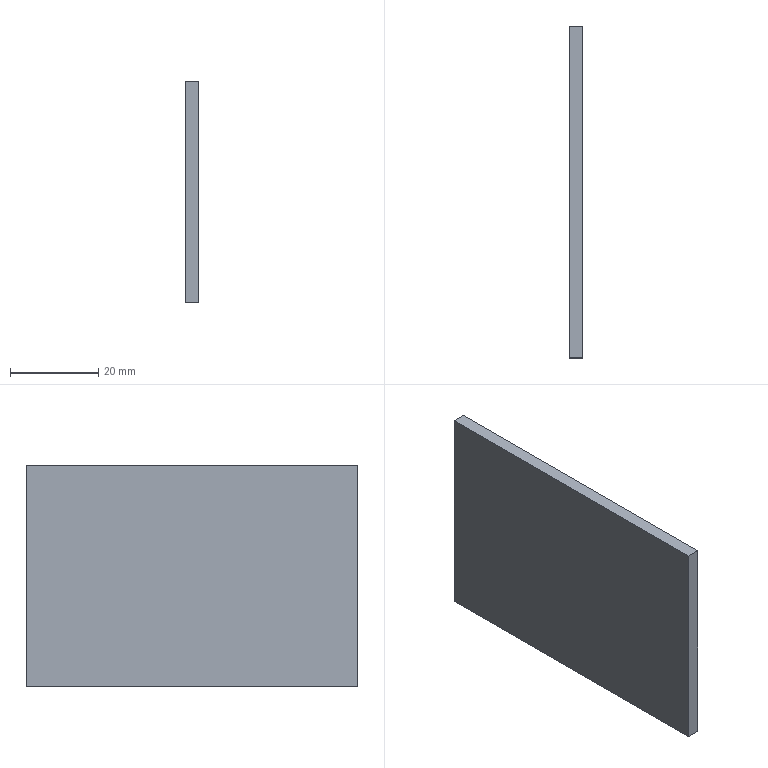Part | STEP file | Positioning_id1486_x_t | 1 solid | 6 faces | box 3 x 75 x 50 mm | volume 11250 mm3 | plane 6
STEP:
#1=CARTESIAN_POINT('',(0.,0.,0.));
#2=DIRECTION('',(0.,0.,1.));
#3=DIRECTION('',(1.,0.,0.));
#4=AXIS2_PLACEMENT_3D('',#1,#2,#3);
#5=CARTESIAN_POINT('',(-1013.002,-37.5,133.532));
#6=VERTEX_POINT('',#5);
#7=CARTESIAN_POINT('',(-1010.002,-37.5,133.532));
#8=VERTEX_POINT('',#7);
#9=CARTESIAN_POINT('',(-1013.002,-37.5,133.532));
#10=DIRECTION('',(1.,0.,0.));
#11=VECTOR('',#10,1.);
#12=LINE('',#9,#11);
#13=CARTESIAN_POINT('',(-1015.002,-37.5,143.532));
#14=DIRECTION('',(0.,-1.,0.));
#15=DIRECTION('',(1.,0.,0.));
#16=AXIS2_PLACEMENT_3D('',#13,#14,#15);
#17=PLANE('',#16);
#18=CARTESIAN_POINT('',(2.,-10.));
#19=DIRECTION('',(1.,0.));
#20=VECTOR('',#19,1.);
#21=LINE('',#18,#20);
#22=(GEOMETRIC_REPRESENTATION_CONTEXT(2)PARAMETRIC_REPRESENTATION_CONTEXT()REPRESENTATION_CONTEXT('',''));
#23=DEFINITIONAL_REPRESENTATION('',(#21),#22);
#24=PCURVE('',#17,#23);
#25=CARTESIAN_POINT('',(-1015.002,2.5,133.532));
#26=DIRECTION('',(0.,0.,-1.));
#27=DIRECTION('',(1.,0.,0.));
#28=AXIS2_PLACEMENT_3D('',#25,#26,#27);
#29=PLANE('',#28);
#30=CARTESIAN_POINT('',(2.,40.));
#31=DIRECTION('',(1.,0.));
#32=VECTOR('',#31,1.);
#33=LINE('',#30,#32);
#34=(GEOMETRIC_REPRESENTATION_CONTEXT(2)PARAMETRIC_REPRESENTATION_CONTEXT()REPRESENTATION_CONTEXT('',''));
#35=DEFINITIONAL_REPRESENTATION('',(#33),#34);
#36=PCURVE('',#29,#35);
#37=SURFACE_CURVE('',#12,(#24,#36),.PCURVE_S1.);
#38=EDGE_CURVE('',#6,#8,#37,.T.);
#39=ORIENTED_EDGE('',*,*,#38,.T.);
#40=CARTESIAN_POINT('',(-1010.002,-37.5,183.532));
#41=VERTEX_POINT('',#40);
#42=CARTESIAN_POINT('',(-1010.002,-37.5,133.532));
#43=DIRECTION('',(0.,0.,1.));
#44=VECTOR('',#43,1.);
#45=LINE('',#42,#44);
#46=CARTESIAN_POINT('',(5.,-10.));
#47=DIRECTION('',(0.,1.));
#48=VECTOR('',#47,1.);
#49=LINE('',#46,#48);
#50=(GEOMETRIC_REPRESENTATION_CONTEXT(2)PARAMETRIC_REPRESENTATION_CONTEXT()REPRESENTATION_CONTEXT('',''));
#51=DEFINITIONAL_REPRESENTATION('',(#49),#50);
#52=PCURVE('',#17,#51);
#53=CARTESIAN_POINT('',(-1010.002,-37.5,133.532));
#54=DIRECTION('',(1.,0.,0.));
#55=DIRECTION('',(0.,0.,1.));
#56=AXIS2_PLACEMENT_3D('',#53,#54,#55);
#57=PLANE('',#56);
#58=CARTESIAN_POINT('',(0.,0.));
#59=DIRECTION('',(1.,0.));
#60=VECTOR('',#59,1.);
#61=LINE('',#58,#60);
#62=(GEOMETRIC_REPRESENTATION_CONTEXT(2)PARAMETRIC_REPRESENTATION_CONTEXT()REPRESENTATION_CONTEXT('',''));
#63=DEFINITIONAL_REPRESENTATION('',(#61),#62);
#64=PCURVE('',#57,#63);
#65=SURFACE_CURVE('',#45,(#52,#64),.PCURVE_S1.);
#66=EDGE_CURVE('',#8,#41,#65,.T.);
#67=ORIENTED_EDGE('',*,*,#66,.T.);
#68=CARTESIAN_POINT('',(-1013.002,-37.5,183.532));
#69=VERTEX_POINT('',#68);
#70=CARTESIAN_POINT('',(-1013.002,-37.5,183.532));
#71=DIRECTION('',(1.,0.,0.));
#72=VECTOR('',#71,1.);
#73=LINE('',#70,#72);
#74=CARTESIAN_POINT('',(2.,40.));
#75=DIRECTION('',(1.,0.));
#76=VECTOR('',#75,1.);
#77=LINE('',#74,#76);
#78=(GEOMETRIC_REPRESENTATION_CONTEXT(2)PARAMETRIC_REPRESENTATION_CONTEXT()REPRESENTATION_CONTEXT('',''));
#79=DEFINITIONAL_REPRESENTATION('',(#77),#78);
#80=PCURVE('',#17,#79);
#81=CARTESIAN_POINT('',(-1015.002,2.5,183.532));
#82=DIRECTION('',(0.,0.,1.));
#83=DIRECTION('',(-1.,0.,0.));
#84=AXIS2_PLACEMENT_3D('',#81,#82,#83);
#85=PLANE('',#84);
#86=CARTESIAN_POINT('',(-2.,40.));
#87=DIRECTION('',(-1.,0.));
#88=VECTOR('',#87,1.);
#89=LINE('',#86,#88);
#90=(GEOMETRIC_REPRESENTATION_CONTEXT(2)PARAMETRIC_REPRESENTATION_CONTEXT()REPRESENTATION_CONTEXT('',''));
#91=DEFINITIONAL_REPRESENTATION('',(#89),#90);
#92=PCURVE('',#85,#91);
#93=SURFACE_CURVE('',#73,(#80,#92),.PCURVE_S1.);
#94=EDGE_CURVE('',#69,#41,#93,.T.);
#95=ORIENTED_EDGE('',*,*,#94,.F.);
#96=CARTESIAN_POINT('',(-1013.002,-37.5,183.532));
#97=DIRECTION('',(0.,0.,-1.));
#98=VECTOR('',#97,1.);
#99=LINE('',#96,#98);
#100=CARTESIAN_POINT('',(2.,40.));
#101=DIRECTION('',(0.,-1.));
#102=VECTOR('',#101,1.);
#103=LINE('',#100,#102);
#104=(GEOMETRIC_REPRESENTATION_CONTEXT(2)PARAMETRIC_REPRESENTATION_CONTEXT()REPRESENTATION_CONTEXT('',''));
#105=DEFINITIONAL_REPRESENTATION('',(#103),#104);
#106=PCURVE('',#17,#105);
#107=CARTESIAN_POINT('',(-1013.002,2.5,143.532));
#108=DIRECTION('',(-1.,0.,0.));
#109=DIRECTION('',(0.,0.,-1.));
#110=AXIS2_PLACEMENT_3D('',#107,#108,#109);
#111=PLANE('',#110);
#112=CARTESIAN_POINT('',(-40.,40.));
#113=DIRECTION('',(1.,0.));
#114=VECTOR('',#113,1.);
#115=LINE('',#112,#114);
#116=(GEOMETRIC_REPRESENTATION_CONTEXT(2)PARAMETRIC_REPRESENTATION_CONTEXT()REPRESENTATION_CONTEXT('',''));
#117=DEFINITIONAL_REPRESENTATION('',(#115),#116);
#118=PCURVE('',#111,#117);
#119=SURFACE_CURVE('',#99,(#106,#118),.PCURVE_S1.);
#120=EDGE_CURVE('',#69,#6,#119,.T.);
#121=ORIENTED_EDGE('',*,*,#120,.T.);
#122=EDGE_LOOP('',(#39,#67,#95,#121));
#123=FACE_BOUND('',#122,.T.);
#124=ADVANCED_FACE('',(#123),#17,.T.);
#125=ORIENTED_EDGE('',*,*,#94,.T.);
#126=CARTESIAN_POINT('',(-1010.002,37.5,183.532));
#127=VERTEX_POINT('',#126);
#128=CARTESIAN_POINT('',(-1010.002,-37.5,183.532));
#129=DIRECTION('',(0.,1.,0.));
#130=VECTOR('',#129,1.);
#131=LINE('',#128,#130);
#132=CARTESIAN_POINT('',(-5.,40.));
#133=DIRECTION('',(0.,-1.));
#134=VECTOR('',#133,1.);
#135=LINE('',#132,#134);
#136=(GEOMETRIC_REPRESENTATION_CONTEXT(2)PARAMETRIC_REPRESENTATION_CONTEXT()REPRESENTATION_CONTEXT('',''));
#137=DEFINITIONAL_REPRESENTATION('',(#135),#136);
#138=PCURVE('',#85,#137);
#139=CARTESIAN_POINT('',(50.,0.));
#140=DIRECTION('',(0.,-1.));
#141=VECTOR('',#140,1.);
#142=LINE('',#139,#141);
#143=(GEOMETRIC_REPRESENTATION_CONTEXT(2)PARAMETRIC_REPRESENTATION_CONTEXT()REPRESENTATION_CONTEXT('',''));
#144=DEFINITIONAL_REPRESENTATION('',(#142),#143);
#145=PCURVE('',#57,#144);
#146=SURFACE_CURVE('',#131,(#138,#145),.PCURVE_S1.);
#147=EDGE_CURVE('',#41,#127,#146,.T.);
#148=ORIENTED_EDGE('',*,*,#147,.T.);
#149=CARTESIAN_POINT('',(-1013.002,37.5,183.532));
#150=VERTEX_POINT('',#149);
#151=CARTESIAN_POINT('',(-1013.002,37.5,183.532));
#152=DIRECTION('',(1.,0.,0.));
#153=VECTOR('',#152,1.);
#154=LINE('',#151,#153);
#155=CARTESIAN_POINT('',(-2.,-35.));
#156=DIRECTION('',(-1.,0.));
#157=VECTOR('',#156,1.);
#158=LINE('',#155,#157);
#159=(GEOMETRIC_REPRESENTATION_CONTEXT(2)PARAMETRIC_REPRESENTATION_CONTEXT()REPRESENTATION_CONTEXT('',''));
#160=DEFINITIONAL_REPRESENTATION('',(#158),#159);
#161=PCURVE('',#85,#160);
#162=CARTESIAN_POINT('',(-1015.002,37.5,143.532));
#163=DIRECTION('',(0.,1.,0.));
#164=DIRECTION('',(-1.,0.,0.));
#165=AXIS2_PLACEMENT_3D('',#162,#163,#164);
#166=PLANE('',#165);
#167=CARTESIAN_POINT('',(-2.,40.));
#168=DIRECTION('',(-1.,0.));
#169=VECTOR('',#168,1.);
#170=LINE('',#167,#169);
#171=(GEOMETRIC_REPRESENTATION_CONTEXT(2)PARAMETRIC_REPRESENTATION_CONTEXT()REPRESENTATION_CONTEXT('',''));
#172=DEFINITIONAL_REPRESENTATION('',(#170),#171);
#173=PCURVE('',#166,#172);
#174=SURFACE_CURVE('',#154,(#161,#173),.PCURVE_S1.);
#175=EDGE_CURVE('',#150,#127,#174,.T.);
#176=ORIENTED_EDGE('',*,*,#175,.F.);
#177=CARTESIAN_POINT('',(-1013.002,37.5,183.532));
#178=DIRECTION('',(0.,-1.,0.));
#179=VECTOR('',#178,1.);
#180=LINE('',#177,#179);
#181=CARTESIAN_POINT('',(-2.,-35.));
#182=DIRECTION('',(0.,1.));
#183=VECTOR('',#182,1.);
#184=LINE('',#181,#183);
#185=(GEOMETRIC_REPRESENTATION_CONTEXT(2)PARAMETRIC_REPRESENTATION_CONTEXT()REPRESENTATION_CONTEXT('',''));
#186=DEFINITIONAL_REPRESENTATION('',(#184),#185);
#187=PCURVE('',#85,#186);
#188=CARTESIAN_POINT('',(-40.,-35.));
#189=DIRECTION('',(0.,1.));
#190=VECTOR('',#189,1.);
#191=LINE('',#188,#190);
#192=(GEOMETRIC_REPRESENTATION_CONTEXT(2)PARAMETRIC_REPRESENTATION_CONTEXT()REPRESENTATION_CONTEXT('',''));
#193=DEFINITIONAL_REPRESENTATION('',(#191),#192);
#194=PCURVE('',#111,#193);
#195=SURFACE_CURVE('',#180,(#187,#194),.PCURVE_S1.);
#196=EDGE_CURVE('',#150,#69,#195,.T.);
#197=ORIENTED_EDGE('',*,*,#196,.T.);
#198=EDGE_LOOP('',(#125,#148,#176,#197));
#199=FACE_BOUND('',#198,.T.);
#200=ADVANCED_FACE('',(#199),#85,.T.);
#201=ORIENTED_EDGE('',*,*,#175,.T.);
#202=CARTESIAN_POINT('',(-1010.002,37.5,133.532));
#203=VERTEX_POINT('',#202);
#204=CARTESIAN_POINT('',(-1010.002,37.5,183.532));
#205=DIRECTION('',(0.,0.,-1.));
#206=VECTOR('',#205,1.);
#207=LINE('',#204,#206);
#208=CARTESIAN_POINT('',(-5.,40.));
#209=DIRECTION('',(0.,-1.));
#210=VECTOR('',#209,1.);
#211=LINE('',#208,#210);
#212=(GEOMETRIC_REPRESENTATION_CONTEXT(2)PARAMETRIC_REPRESENTATION_CONTEXT()REPRESENTATION_CONTEXT('',''));
#213=DEFINITIONAL_REPRESENTATION('',(#211),#212);
#214=PCURVE('',#166,#213);
#215=CARTESIAN_POINT('',(50.,-75.));
#216=DIRECTION('',(-1.,0.));
#217=VECTOR('',#216,1.);
#218=LINE('',#215,#217);
#219=(GEOMETRIC_REPRESENTATION_CONTEXT(2)PARAMETRIC_REPRESENTATION_CONTEXT()REPRESENTATION_CONTEXT('',''));
#220=DEFINITIONAL_REPRESENTATION('',(#218),#219);
#221=PCURVE('',#57,#220);
#222=SURFACE_CURVE('',#207,(#214,#221),.PCURVE_S1.);
#223=EDGE_CURVE('',#127,#203,#222,.T.);
#224=ORIENTED_EDGE('',*,*,#223,.T.);
#225=CARTESIAN_POINT('',(-1013.002,37.5,133.532));
#226=VERTEX_POINT('',#225);
#227=CARTESIAN_POINT('',(-1013.002,37.5,133.532));
#228=DIRECTION('',(1.,0.,0.));
#229=VECTOR('',#228,1.);
#230=LINE('',#227,#229);
#231=CARTESIAN_POINT('',(-2.,-10.));
#232=DIRECTION('',(-1.,0.));
#233=VECTOR('',#232,1.);
#234=LINE('',#231,#233);
#235=(GEOMETRIC_REPRESENTATION_CONTEXT(2)PARAMETRIC_REPRESENTATION_CONTEXT()REPRESENTATION_CONTEXT('',''));
#236=DEFINITIONAL_REPRESENTATION('',(#234),#235);
#237=PCURVE('',#166,#236);
#238=CARTESIAN_POINT('',(2.,-35.));
#239=DIRECTION('',(1.,0.));
#240=VECTOR('',#239,1.);
#241=LINE('',#238,#240);
#242=(GEOMETRIC_REPRESENTATION_CONTEXT(2)PARAMETRIC_REPRESENTATION_CONTEXT()REPRESENTATION_CONTEXT('',''));
#243=DEFINITIONAL_REPRESENTATION('',(#241),#242);
#244=PCURVE('',#29,#243);
#245=SURFACE_CURVE('',#230,(#237,#244),.PCURVE_S1.);
#246=EDGE_CURVE('',#226,#203,#245,.T.);
#247=ORIENTED_EDGE('',*,*,#246,.F.);
#248=CARTESIAN_POINT('',(-1013.002,37.5,133.532));
#249=DIRECTION('',(0.,0.,1.));
#250=VECTOR('',#249,1.);
#251=LINE('',#248,#250);
#252=CARTESIAN_POINT('',(-2.,-10.));
#253=DIRECTION('',(0.,1.));
#254=VECTOR('',#253,1.);
#255=LINE('',#252,#254);
#256=(GEOMETRIC_REPRESENTATION_CONTEXT(2)PARAMETRIC_REPRESENTATION_CONTEXT()REPRESENTATION_CONTEXT('',''));
#257=DEFINITIONAL_REPRESENTATION('',(#255),#256);
#258=PCURVE('',#166,#257);
#259=CARTESIAN_POINT('',(10.,-35.));
#260=DIRECTION('',(-1.,0.));
#261=VECTOR('',#260,1.);
#262=LINE('',#259,#261);
#263=(GEOMETRIC_REPRESENTATION_CONTEXT(2)PARAMETRIC_REPRESENTATION_CONTEXT()REPRESENTATION_CONTEXT('',''));
#264=DEFINITIONAL_REPRESENTATION('',(#262),#263);
#265=PCURVE('',#111,#264);
#266=SURFACE_CURVE('',#251,(#258,#265),.PCURVE_S1.);
#267=EDGE_CURVE('',#226,#150,#266,.T.);
#268=ORIENTED_EDGE('',*,*,#267,.T.);
#269=EDGE_LOOP('',(#201,#224,#247,#268));
#270=FACE_BOUND('',#269,.T.);
#271=ADVANCED_FACE('',(#270),#166,.T.);
#272=ORIENTED_EDGE('',*,*,#246,.T.);
#273=CARTESIAN_POINT('',(-1010.002,37.5,133.532));
#274=DIRECTION('',(0.,-1.,0.));
#275=VECTOR('',#274,1.);
#276=LINE('',#273,#275);
#277=CARTESIAN_POINT('',(5.,-35.));
#278=DIRECTION('',(0.,1.));
#279=VECTOR('',#278,1.);
#280=LINE('',#277,#279);
#281=(GEOMETRIC_REPRESENTATION_CONTEXT(2)PARAMETRIC_REPRESENTATION_CONTEXT()REPRESENTATION_CONTEXT('',''));
#282=DEFINITIONAL_REPRESENTATION('',(#280),#281);
#283=PCURVE('',#29,#282);
#284=CARTESIAN_POINT('',(0.,-75.));
#285=DIRECTION('',(0.,1.));
#286=VECTOR('',#285,1.);
#287=LINE('',#284,#286);
#288=(GEOMETRIC_REPRESENTATION_CONTEXT(2)PARAMETRIC_REPRESENTATION_CONTEXT()REPRESENTATION_CONTEXT('',''));
#289=DEFINITIONAL_REPRESENTATION('',(#287),#288);
#290=PCURVE('',#57,#289);
#291=SURFACE_CURVE('',#276,(#283,#290),.PCURVE_S1.);
#292=EDGE_CURVE('',#203,#8,#291,.T.);
#293=ORIENTED_EDGE('',*,*,#292,.T.);
#294=ORIENTED_EDGE('',*,*,#38,.F.);
#295=CARTESIAN_POINT('',(-1013.002,-37.5,133.532));
#296=DIRECTION('',(0.,1.,0.));
#297=VECTOR('',#296,1.);
#298=LINE('',#295,#297);
#299=CARTESIAN_POINT('',(2.,40.));
#300=DIRECTION('',(0.,-1.));
#301=VECTOR('',#300,1.);
#302=LINE('',#299,#301);
#303=(GEOMETRIC_REPRESENTATION_CONTEXT(2)PARAMETRIC_REPRESENTATION_CONTEXT()REPRESENTATION_CONTEXT('',''));
#304=DEFINITIONAL_REPRESENTATION('',(#302),#303);
#305=PCURVE('',#29,#304);
#306=CARTESIAN_POINT('',(10.,40.));
#307=DIRECTION('',(0.,-1.));
#308=VECTOR('',#307,1.);
#309=LINE('',#306,#308);
#310=(GEOMETRIC_REPRESENTATION_CONTEXT(2)PARAMETRIC_REPRESENTATION_CONTEXT()REPRESENTATION_CONTEXT('',''));
#311=DEFINITIONAL_REPRESENTATION('',(#309),#310);
#312=PCURVE('',#111,#311);
#313=SURFACE_CURVE('',#298,(#305,#312),.PCURVE_S1.);
#314=EDGE_CURVE('',#6,#226,#313,.T.);
#315=ORIENTED_EDGE('',*,*,#314,.T.);
#316=EDGE_LOOP('',(#272,#293,#294,#315));
#317=FACE_BOUND('',#316,.T.);
#318=ADVANCED_FACE('',(#317),#29,.T.);
#319=ORIENTED_EDGE('',*,*,#314,.F.);
#320=ORIENTED_EDGE('',*,*,#120,.F.);
#321=ORIENTED_EDGE('',*,*,#196,.F.);
#322=ORIENTED_EDGE('',*,*,#267,.F.);
#323=EDGE_LOOP('',(#319,#320,#321,#322));
#324=FACE_BOUND('',#323,.T.);
#325=ADVANCED_FACE('',(#324),#111,.T.);
#326=ORIENTED_EDGE('',*,*,#66,.F.);
#327=ORIENTED_EDGE('',*,*,#292,.F.);
#328=ORIENTED_EDGE('',*,*,#223,.F.);
#329=ORIENTED_EDGE('',*,*,#147,.F.);
#330=EDGE_LOOP('',(#326,#327,#328,#329));
#331=FACE_BOUND('',#330,.T.);
#332=ADVANCED_FACE('',(#331),#57,.T.);
#333=CLOSED_SHELL('',(#124,#200,#271,#318,#325,#332));
#334=MANIFOLD_SOLID_BREP('',#333);
#335=(LENGTH_UNIT()NAMED_UNIT(*)SI_UNIT(.MILLI.,.METRE.));
#336=UNCERTAINTY_MEASURE_WITH_UNIT(LENGTH_MEASURE(0.0000001),#335,'','');
#337=(NAMED_UNIT(*)PLANE_ANGLE_UNIT()SI_UNIT($,.RADIAN.));
#338=(NAMED_UNIT(*)SI_UNIT($,.STERADIAN.)SOLID_ANGLE_UNIT());
#339=(GEOMETRIC_REPRESENTATION_CONTEXT(3)GLOBAL_UNCERTAINTY_ASSIGNED_CONTEXT((#336))GLOBAL_UNIT_ASSIGNED_CONTEXT((#335,#337,#338))REPRESENTATION_CONTEXT('',''));
#340=ADVANCED_BREP_SHAPE_REPRESENTATION('',(#4,#334),#339);